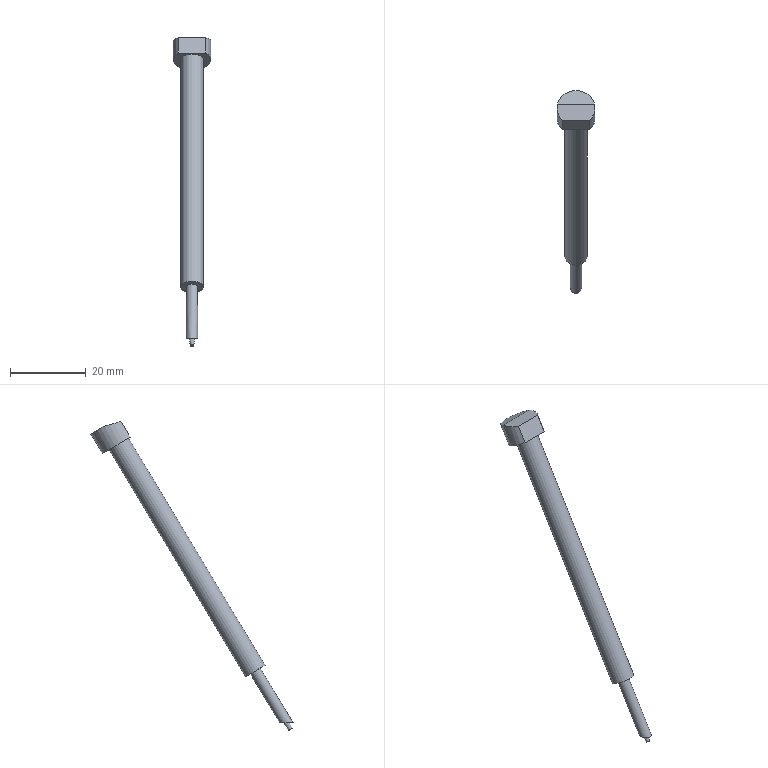Part | STEP file | lll_id30_x_t | 1 solid | 11 faces | box 10 x 53.41 x 81.544 mm | volume 2497 mm3 | plane 7 | cylinder 3 | cone 1 | commonest cylinder face diameters 3 x1 6 x1 10 x1
STEP:
#1=CARTESIAN_POINT('',(-4.924,85.966,120.145));
#2=VERTEX_POINT('',#1);
#3=CARTESIAN_POINT('',(-3.571,81.575,121.322));
#4=VERTEX_POINT('',#3);
#5=CARTESIAN_POINT('',(0.00001281,85.092,120.38));
#6=DIRECTION('',(0.,0.2588,0.9659));
#7=DIRECTION('',(0.,0.9659,-0.2588));
#8=AXIS2_PLACEMENT_3D('',#5,#6,#7);
#9=ELLIPSE('',#8,5.201,5.);
#10=EDGE_CURVE('',#2,#4,#9,.T.);
#11=ORIENTED_EDGE('',*,*,#10,.F.);
#12=CARTESIAN_POINT('',(4.924,85.966,120.145));
#13=VERTEX_POINT('',#12);
#14=CARTESIAN_POINT('',(0.00001281,85.22,120.593));
#15=DIRECTION('',(0.,0.515,0.8572));
#16=DIRECTION('',(0.,-0.8572,0.515));
#17=AXIS2_PLACEMENT_3D('',#14,#15,#16);
#18=CIRCLE('',#17,5.);
#19=EDGE_CURVE('',#13,#2,#18,.T.);
#20=ORIENTED_EDGE('',*,*,#19,.F.);
#21=CARTESIAN_POINT('',(3.571,81.575,121.322));
#22=VERTEX_POINT('',#21);
#23=CARTESIAN_POINT('',(0.00001281,85.092,120.38));
#24=DIRECTION('',(0.,0.2588,0.9659));
#25=DIRECTION('',(0.,0.9659,-0.2588));
#26=AXIS2_PLACEMENT_3D('',#23,#24,#25);
#27=ELLIPSE('',#26,5.201,5.);
#28=EDGE_CURVE('',#22,#13,#27,.T.);
#29=ORIENTED_EDGE('',*,*,#28,.F.);
#30=CARTESIAN_POINT('',(3.571,79.13,117.253));
#31=VERTEX_POINT('',#30);
#32=CARTESIAN_POINT('',(3.571,43.077,57.251));
#33=DIRECTION('',(0.,0.515,0.8572));
#34=VECTOR('',#33,1.);
#35=LINE('',#32,#34);
#36=EDGE_CURVE('',#31,#22,#35,.T.);
#37=ORIENTED_EDGE('',*,*,#36,.F.);
#38=CARTESIAN_POINT('',(-3.571,79.13,117.253));
#39=VERTEX_POINT('',#38);
#40=CARTESIAN_POINT('',(0.00001281,82.13,115.45));
#41=DIRECTION('',(0.,-0.515,-0.8572));
#42=DIRECTION('',(0.,-0.8572,0.515));
#43=AXIS2_PLACEMENT_3D('',#40,#41,#42);
#44=CIRCLE('',#43,5.);
#45=EDGE_CURVE('',#39,#31,#44,.T.);
#46=ORIENTED_EDGE('',*,*,#45,.F.);
#47=CARTESIAN_POINT('',(-3.571,43.077,57.251));
#48=DIRECTION('',(0.,-0.515,-0.8572));
#49=VECTOR('',#48,1.);
#50=LINE('',#47,#49);
#51=EDGE_CURVE('',#4,#39,#50,.T.);
#52=ORIENTED_EDGE('',*,*,#51,.F.);
#53=EDGE_LOOP('',(#11,#20,#29,#37,#46,#52));
#54=FACE_OUTER_BOUND('',#53,.T.);
#55=CARTESIAN_POINT('',(0.00001281,46.077,55.449));
#56=DIRECTION('',(0.,0.515,0.8572));
#57=DIRECTION('',(0.,-0.8572,0.515));
#58=AXIS2_PLACEMENT_3D('',#55,#56,#57);
#59=CYLINDRICAL_SURFACE('',#58,5.);
#60=ADVANCED_FACE('',(#54),#59,.T.);
#61=ORIENTED_EDGE('',*,*,#19,.T.);
#62=CARTESIAN_POINT('',(0.00001281,85.966,120.145));
#63=DIRECTION('',(1.,0.,0.));
#64=VECTOR('',#63,1.);
#65=LINE('',#62,#64);
#66=EDGE_CURVE('',#2,#13,#65,.T.);
#67=ORIENTED_EDGE('',*,*,#66,.T.);
#68=EDGE_LOOP('',(#61,#67));
#69=FACE_OUTER_BOUND('',#68,.T.);
#70=CARTESIAN_POINT('',(0.00001281,85.22,120.593));
#71=DIRECTION('',(0.,0.515,0.8572));
#72=DIRECTION('',(0.,-0.8572,0.515));
#73=AXIS2_PLACEMENT_3D('',#70,#71,#72);
#74=PLANE('',#73);
#75=ADVANCED_FACE('',(#69),#74,.T.);
#76=ORIENTED_EDGE('',*,*,#36,.T.);
#77=CARTESIAN_POINT('',(0.00001281,81.575,121.322));
#78=DIRECTION('',(-1.,0.,0.));
#79=VECTOR('',#78,1.);
#80=LINE('',#77,#79);
#81=EDGE_CURVE('',#22,#4,#80,.T.);
#82=ORIENTED_EDGE('',*,*,#81,.T.);
#83=ORIENTED_EDGE('',*,*,#51,.T.);
#84=CARTESIAN_POINT('',(0.00001281,79.13,117.253));
#85=DIRECTION('',(1.,0.,0.));
#86=VECTOR('',#85,1.);
#87=LINE('',#84,#86);
#88=EDGE_CURVE('',#39,#31,#87,.T.);
#89=ORIENTED_EDGE('',*,*,#88,.T.);
#90=EDGE_LOOP('',(#76,#82,#83,#89));
#91=FACE_OUTER_BOUND('',#90,.T.);
#92=CARTESIAN_POINT('',(0.00001281,78.1,115.539));
#93=DIRECTION('',(0.,-0.8572,0.515));
#94=DIRECTION('',(0.,-0.515,-0.8572));
#95=AXIS2_PLACEMENT_3D('',#92,#93,#94);
#96=PLANE('',#95);
#97=ADVANCED_FACE('',(#91),#96,.T.);
#98=CARTESIAN_POINT('',(0.00001281,79.559,116.996));
#99=VERTEX_POINT('',#98);
#100=CARTESIAN_POINT('',(0.00001281,82.13,115.45));
#101=DIRECTION('',(0.,-0.515,-0.8572));
#102=DIRECTION('',(0.,-0.8572,0.515));
#103=AXIS2_PLACEMENT_3D('',#100,#101,#102);
#104=CIRCLE('',#103,3.);
#105=EDGE_CURVE('',#99,#99,#104,.T.);
#106=ORIENTED_EDGE('',*,*,#105,.F.);
#107=EDGE_LOOP('',(#106));
#108=FACE_BOUND('',#107,.T.);
#109=ORIENTED_EDGE('',*,*,#88,.F.);
#110=ORIENTED_EDGE('',*,*,#45,.T.);
#111=EDGE_LOOP('',(#109,#110));
#112=FACE_BOUND('',#111,.T.);
#113=CARTESIAN_POINT('',(0.00001281,82.344,115.322));
#114=DIRECTION('',(0.,0.515,0.8572));
#115=DIRECTION('',(0.,-0.8572,0.515));
#116=AXIS2_PLACEMENT_3D('',#113,#114,#115);
#117=PLANE('',#116);
#118=ADVANCED_FACE('',(#108,#112),#117,.F.);
#119=CARTESIAN_POINT('',(0.00001281,43.506,56.994));
#120=VERTEX_POINT('',#119);
#121=CARTESIAN_POINT('',(0.00001281,46.077,55.449));
#122=DIRECTION('',(0.,0.515,0.8572));
#123=DIRECTION('',(0.,-0.8572,0.515));
#124=AXIS2_PLACEMENT_3D('',#121,#122,#123);
#125=CIRCLE('',#124,3.);
#126=EDGE_CURVE('',#120,#120,#125,.T.);
#127=ORIENTED_EDGE('',*,*,#126,.T.);
#128=EDGE_LOOP('',(#127));
#129=FACE_BOUND('',#128,.T.);
#130=ORIENTED_EDGE('',*,*,#105,.T.);
#131=EDGE_LOOP('',(#130));
#132=FACE_BOUND('',#131,.T.);
#133=CARTESIAN_POINT('',(0.00001281,46.077,55.449));
#134=DIRECTION('',(0.,0.515,0.8572));
#135=DIRECTION('',(0.,-0.8572,0.515));
#136=AXIS2_PLACEMENT_3D('',#133,#134,#135);
#137=CYLINDRICAL_SURFACE('',#136,3.);
#138=ADVANCED_FACE('',(#129,#132),#137,.T.);
#139=CARTESIAN_POINT('',(0.00001281,47.363,54.676));
#140=VERTEX_POINT('',#139);
#141=CARTESIAN_POINT('',(0.00001281,46.077,55.449));
#142=DIRECTION('',(0.,-0.515,-0.8572));
#143=DIRECTION('',(0.,0.8572,-0.515));
#144=AXIS2_PLACEMENT_3D('',#141,#142,#143);
#145=CIRCLE('',#144,1.5);
#146=EDGE_CURVE('',#140,#140,#145,.T.);
#147=ORIENTED_EDGE('',*,*,#146,.T.);
#148=EDGE_LOOP('',(#147));
#149=FACE_BOUND('',#148,.T.);
#150=CARTESIAN_POINT('',(0.00001281,39.596,41.75));
#151=VERTEX_POINT('',#150);
#152=CARTESIAN_POINT('',(0.00001281,37.846,41.75));
#153=DIRECTION('',(0.,0.,1.));
#154=DIRECTION('',(0.,1.,0.));
#155=AXIS2_PLACEMENT_3D('',#152,#153,#154);
#156=ELLIPSE('',#155,1.75,1.5);
#157=EDGE_CURVE('',#151,#151,#156,.T.);
#158=ORIENTED_EDGE('',*,*,#157,.T.);
#159=EDGE_LOOP('',(#158));
#160=FACE_BOUND('',#159,.T.);
#161=CARTESIAN_POINT('',(0.00001281,311.322,496.89));
#162=DIRECTION('',(0.,-0.515,-0.8572));
#163=DIRECTION('',(0.,0.8572,-0.515));
#164=AXIS2_PLACEMENT_3D('',#161,#162,#163);
#165=CYLINDRICAL_SURFACE('',#164,1.5);
#166=ADVANCED_FACE('',(#149,#160),#165,.T.);
#167=CARTESIAN_POINT('',(0.00001281,37.245,39.778));
#168=VERTEX_POINT('',#167);
#169=CARTESIAN_POINT('',(0.00001281,36.816,40.036));
#170=DIRECTION('',(0.,0.515,0.8572));
#171=DIRECTION('',(0.,0.8572,-0.515));
#172=AXIS2_PLACEMENT_3D('',#169,#170,#171);
#173=CIRCLE('',#172,0.5);
#174=EDGE_CURVE('',#168,#168,#173,.T.);
#175=ORIENTED_EDGE('',*,*,#174,.F.);
#176=EDGE_LOOP('',(#175));
#177=FACE_OUTER_BOUND('',#176,.T.);
#178=CARTESIAN_POINT('',(0.00001281,36.816,40.036));
#179=DIRECTION('',(0.,-0.515,-0.8572));
#180=DIRECTION('',(0.,0.8572,-0.515));
#181=AXIS2_PLACEMENT_3D('',#178,#179,#180);
#182=PLANE('',#181);
#183=ADVANCED_FACE('',(#177),#182,.T.);
#184=ORIENTED_EDGE('',*,*,#174,.T.);
#185=EDGE_LOOP('',(#184));
#186=FACE_BOUND('',#185,.T.);
#187=CARTESIAN_POINT('',(0.00001281,38.678,41.75));
#188=VERTEX_POINT('',#187);
#189=CARTESIAN_POINT('',(0.00001281,37.888,41.75));
#190=DIRECTION('',(0.,0.,1.));
#191=DIRECTION('',(0.,1.,0.));
#192=AXIS2_PLACEMENT_3D('',#189,#190,#191);
#193=ELLIPSE('',#192,0.7896,0.6759);
#194=EDGE_CURVE('',#188,#188,#193,.T.);
#195=ORIENTED_EDGE('',*,*,#194,.F.);
#196=EDGE_LOOP('',(#195));
#197=FACE_BOUND('',#196,.T.);
#198=CARTESIAN_POINT('',(0.00001281,36.816,40.036));
#199=DIRECTION('',(0.,0.515,0.8572));
#200=DIRECTION('',(0.,0.8572,-0.515));
#201=AXIS2_PLACEMENT_3D('',#198,#199,#200);
#202=CONICAL_SURFACE('',#201,0.5,5.);
#203=ADVANCED_FACE('',(#186,#197),#202,.T.);
#204=ORIENTED_EDGE('',*,*,#194,.T.);
#205=EDGE_LOOP('',(#204));
#206=FACE_BOUND('',#205,.T.);
#207=ORIENTED_EDGE('',*,*,#157,.F.);
#208=EDGE_LOOP('',(#207));
#209=FACE_BOUND('',#208,.T.);
#210=CARTESIAN_POINT('',(0.00001281,37.904,41.75));
#211=DIRECTION('',(0.,0.,1.));
#212=DIRECTION('',(0.,1.,0.));
#213=AXIS2_PLACEMENT_3D('',#210,#211,#212);
#214=PLANE('',#213);
#215=ADVANCED_FACE('',(#206,#209),#214,.F.);
#216=ORIENTED_EDGE('',*,*,#126,.F.);
#217=EDGE_LOOP('',(#216));
#218=FACE_BOUND('',#217,.T.);
#219=ORIENTED_EDGE('',*,*,#146,.F.);
#220=EDGE_LOOP('',(#219));
#221=FACE_BOUND('',#220,.T.);
#222=CARTESIAN_POINT('',(0.00001281,46.077,55.449));
#223=DIRECTION('',(0.,-0.515,-0.8572));
#224=DIRECTION('',(0.,0.8572,-0.515));
#225=AXIS2_PLACEMENT_3D('',#222,#223,#224);
#226=PLANE('',#225);
#227=ADVANCED_FACE('',(#218,#221),#226,.T.);
#228=ORIENTED_EDGE('',*,*,#66,.F.);
#229=ORIENTED_EDGE('',*,*,#10,.T.);
#230=ORIENTED_EDGE('',*,*,#81,.F.);
#231=ORIENTED_EDGE('',*,*,#28,.T.);
#232=EDGE_LOOP('',(#228,#229,#230,#231));
#233=FACE_OUTER_BOUND('',#232,.T.);
#234=CARTESIAN_POINT('',(0.00001281,85.092,120.38));
#235=DIRECTION('',(0.,0.2588,0.9659));
#236=DIRECTION('',(0.,-0.9659,0.2588));
#237=AXIS2_PLACEMENT_3D('',#234,#235,#236);
#238=PLANE('',#237);
#239=ADVANCED_FACE('',(#233),#238,.T.);
#240=CLOSED_SHELL('',(#60,#75,#97,#118,#138,#166,#183,#203,#215,#227,#239));
#241=MANIFOLD_SOLID_BREP('',#240);
#242=(LENGTH_UNIT()NAMED_UNIT(*)SI_UNIT(.MILLI.,.METRE.));
#243=UNCERTAINTY_MEASURE_WITH_UNIT(LENGTH_MEASURE(0.00002),#242,'','');
#244=(NAMED_UNIT(*)PLANE_ANGLE_UNIT()SI_UNIT($,.RADIAN.));
#245=PLANE_ANGLE_MEASURE_WITH_UNIT(PLANE_ANGLE_MEASURE(0.01745),#244);
#246=DIMENSIONAL_EXPONENTS(0.,0.,0.,0.,0.,0.,0.);
#247=(CONVERSION_BASED_UNIT('DEGREE',#245)NAMED_UNIT(#246)PLANE_ANGLE_UNIT());
#248=(NAMED_UNIT(*)SI_UNIT($,.STERADIAN.)SOLID_ANGLE_UNIT());
#249=(GEOMETRIC_REPRESENTATION_CONTEXT(3)GLOBAL_UNCERTAINTY_ASSIGNED_CONTEXT((#243))GLOBAL_UNIT_ASSIGNED_CONTEXT((#242,#247,#248))REPRESENTATION_CONTEXT('',''));
#250=ADVANCED_BREP_SHAPE_REPRESENTATION('',(#241),#249);